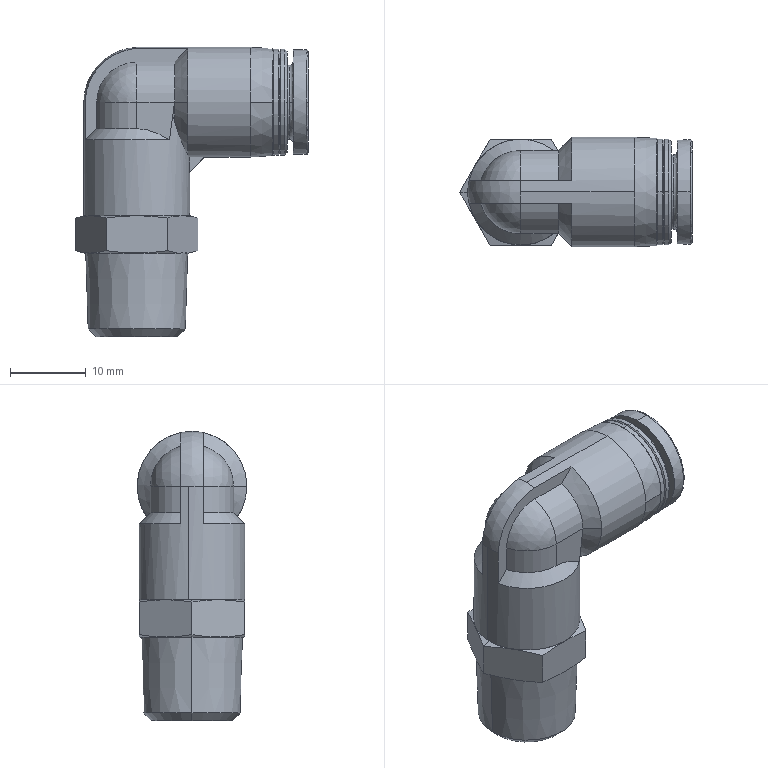Part | NX | 1 solid | 72 faces | box 30.783 x 14.5 x 38.25 mm | volume 6701 mm3 | cone 23 | plane 22 | cylinder 20 | torus 4 | sphere 2 | spline 1 | commonest cylinder face diameters 11 x6 14 x6 8 x2 9.8 x2 13.8 x2 14.5 x2